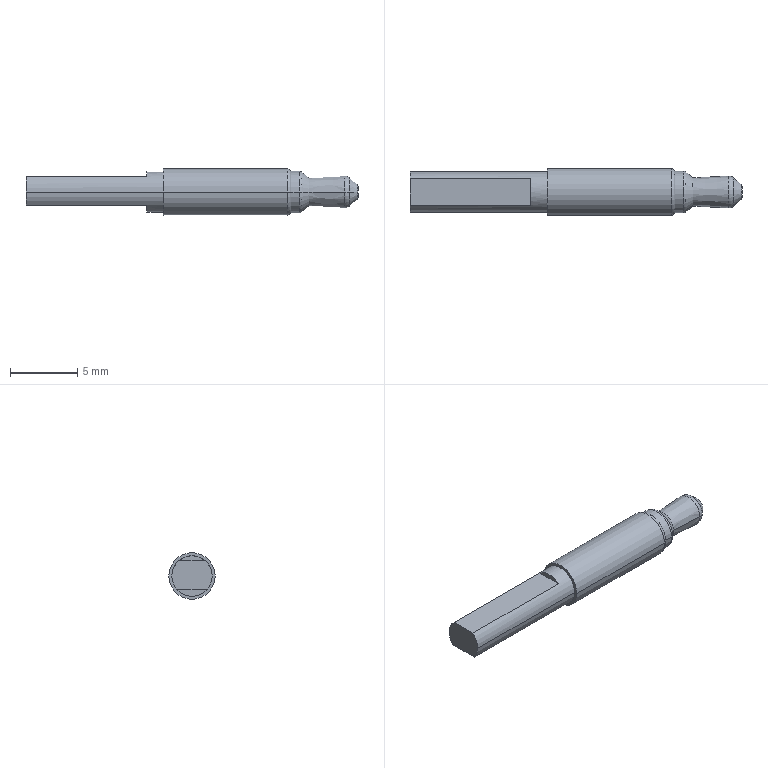Part | NX | 1 solid | 27 faces | box 24.7 x 3.45 x 3.45 mm | volume 170.784 mm3 | torus 8 | plane 7 | cylinder 6 | cone 6 | commonest cylinder face diameters 3 x2 3.1 x2 3.45 x2
STEP:
#1=CARTESIAN_POINT('',(12.641,-1.55,0.));
#2=VERTEX_POINT('',#1);
#3=CARTESIAN_POINT('',(12.641,1.55,0.));
#4=VERTEX_POINT('',#3);
#5=CARTESIAN_POINT('',(12.641,0.,0.));
#6=DIRECTION('',(1.,0.,0.));
#7=DIRECTION('',(0.,-1.,0.));
#8=AXIS2_PLACEMENT_3D('',#5,#6,#7);
#9=CIRCLE('',#8,1.55);
#10=EDGE_CURVE('',#2,#4,#9,.T.);
#11=ORIENTED_EDGE('',*,*,#10,.F.);
#12=CARTESIAN_POINT('',(12.,-1.55,0.));
#13=VERTEX_POINT('',#12);
#14=CARTESIAN_POINT('',(-0.85,-1.55,0.));
#15=DIRECTION('',(1.,0.,0.));
#16=VECTOR('',#15,1000.);
#17=LINE('',#14,#16);
#18=EDGE_CURVE('',#2,#13,#17,.F.);
#19=ORIENTED_EDGE('',*,*,#18,.T.);
#20=CARTESIAN_POINT('',(12.,1.55,0.));
#21=VERTEX_POINT('',#20);
#22=CARTESIAN_POINT('',(12.,0.,0.));
#23=DIRECTION('',(1.,0.,0.));
#24=DIRECTION('',(0.,1.,0.));
#25=AXIS2_PLACEMENT_3D('',#22,#23,#24);
#26=CIRCLE('',#25,1.55);
#27=EDGE_CURVE('',#13,#21,#26,.T.);
#28=ORIENTED_EDGE('',*,*,#27,.T.);
#29=CARTESIAN_POINT('',(-0.85,1.55,0.));
#30=DIRECTION('',(1.,0.,0.));
#31=VECTOR('',#30,1000.);
#32=LINE('',#29,#31);
#33=EDGE_CURVE('',#4,#21,#32,.F.);
#34=ORIENTED_EDGE('',*,*,#33,.F.);
#35=EDGE_LOOP('',(#11,#19,#28,#34));
#36=FACE_BOUND('',#35,.T.);
#37=CARTESIAN_POINT('',(-0.85,0.,0.));
#38=DIRECTION('',(1.,0.,0.));
#39=DIRECTION('',(0.,-1.,0.));
#40=AXIS2_PLACEMENT_3D('',#37,#38,#39);
#41=CYLINDRICAL_SURFACE('',#40,1.55);
#42=ADVANCED_FACE('',(#36),#41,.T.);
#43=CARTESIAN_POINT('',(13.35,-1.05,0.));
#44=VERTEX_POINT('',#43);
#45=CARTESIAN_POINT('',(13.35,1.05,0.));
#46=VERTEX_POINT('',#45);
#47=CARTESIAN_POINT('',(13.35,0.,0.));
#48=DIRECTION('',(1.,0.,0.));
#49=DIRECTION('',(0.,0.,-1.));
#50=AXIS2_PLACEMENT_3D('',#47,#48,#49);
#51=CIRCLE('',#50,1.05);
#52=EDGE_CURVE('',#44,#46,#51,.T.);
#53=ORIENTED_EDGE('',*,*,#52,.F.);
#54=CARTESIAN_POINT('',(12.833,-1.48,0.));
#55=VERTEX_POINT('',#54);
#56=CARTESIAN_POINT('',(13.05,-1.3,0.));
#57=DIRECTION('',(-0.7682,-0.6402,0.));
#58=VECTOR('',#57,1000.);
#59=LINE('',#56,#58);
#60=EDGE_CURVE('',#44,#55,#59,.T.);
#61=ORIENTED_EDGE('',*,*,#60,.T.);
#62=CARTESIAN_POINT('',(12.833,1.48,0.));
#63=VERTEX_POINT('',#62);
#64=CARTESIAN_POINT('',(12.833,0.,0.));
#65=DIRECTION('',(1.,0.,0.));
#66=DIRECTION('',(0.,-1.,0.));
#67=AXIS2_PLACEMENT_3D('',#64,#65,#66);
#68=CIRCLE('',#67,1.48);
#69=EDGE_CURVE('',#55,#63,#68,.T.);
#70=ORIENTED_EDGE('',*,*,#69,.T.);
#71=CARTESIAN_POINT('',(13.05,1.3,0.));
#72=DIRECTION('',(-0.7682,0.6402,0.));
#73=VECTOR('',#72,1000.);
#74=LINE('',#71,#73);
#75=EDGE_CURVE('',#46,#63,#74,.T.);
#76=ORIENTED_EDGE('',*,*,#75,.F.);
#77=EDGE_LOOP('',(#53,#61,#70,#76));
#78=FACE_BOUND('',#77,.T.);
#79=CARTESIAN_POINT('',(13.05,0.,0.));
#80=DIRECTION('',(-1.,0.,0.));
#81=DIRECTION('',(0.,1.,0.));
#82=AXIS2_PLACEMENT_3D('',#79,#80,#81);
#83=CONICAL_SURFACE('',#82,1.3,0.6947);
#84=ADVANCED_FACE('',(#78),#83,.T.);
#85=CARTESIAN_POINT('',(16.932,0.5598,0.));
#86=VERTEX_POINT('',#85);
#87=CARTESIAN_POINT('',(16.932,-0.5598,0.));
#88=VERTEX_POINT('',#87);
#89=CARTESIAN_POINT('',(16.932,0.,0.));
#90=DIRECTION('',(-1.,0.,0.));
#91=DIRECTION('',(0.,-1.,0.));
#92=AXIS2_PLACEMENT_3D('',#89,#90,#91);
#93=CIRCLE('',#92,0.5598);
#94=EDGE_CURVE('',#86,#88,#93,.T.);
#95=ORIENTED_EDGE('',*,*,#94,.T.);
#96=CARTESIAN_POINT('',(16.353,-1.066,0.));
#97=VERTEX_POINT('',#96);
#98=CARTESIAN_POINT('',(16.596,-0.8531,0.));
#99=DIRECTION('',(-0.7526,-0.6585,0.));
#100=VECTOR('',#99,1000.);
#101=LINE('',#98,#100);
#102=EDGE_CURVE('',#88,#97,#101,.T.);
#103=ORIENTED_EDGE('',*,*,#102,.T.);
#104=CARTESIAN_POINT('',(16.353,1.066,0.));
#105=VERTEX_POINT('',#104);
#106=CARTESIAN_POINT('',(16.353,0.,0.));
#107=DIRECTION('',(-1.,0.,0.));
#108=DIRECTION('',(0.,1.,0.));
#109=AXIS2_PLACEMENT_3D('',#106,#107,#108);
#110=CIRCLE('',#109,1.066);
#111=EDGE_CURVE('',#105,#97,#110,.T.);
#112=ORIENTED_EDGE('',*,*,#111,.F.);
#113=CARTESIAN_POINT('',(16.596,0.8531,0.));
#114=DIRECTION('',(-0.7526,0.6585,0.));
#115=VECTOR('',#114,1000.);
#116=LINE('',#113,#115);
#117=EDGE_CURVE('',#86,#105,#116,.T.);
#118=ORIENTED_EDGE('',*,*,#117,.F.);
#119=EDGE_LOOP('',(#95,#103,#112,#118));
#120=FACE_BOUND('',#119,.T.);
#121=CARTESIAN_POINT('',(16.596,0.,0.));
#122=DIRECTION('',(-1.,0.,0.));
#123=DIRECTION('',(0.,1.,0.));
#124=AXIS2_PLACEMENT_3D('',#121,#122,#123);
#125=CONICAL_SURFACE('',#124,0.8531,0.7188);
#126=ADVANCED_FACE('',(#120),#125,.T.);
#127=CARTESIAN_POINT('',(17.,-0.4092,0.));
#128=VERTEX_POINT('',#127);
#129=CARTESIAN_POINT('',(17.,0.4092,0.));
#130=VERTEX_POINT('',#129);
#131=CARTESIAN_POINT('',(17.,0.,0.));
#132=DIRECTION('',(-1.,0.,0.));
#133=DIRECTION('',(0.,1.,0.));
#134=AXIS2_PLACEMENT_3D('',#131,#132,#133);
#135=CIRCLE('',#134,0.4092);
#136=EDGE_CURVE('',#128,#130,#135,.T.);
#137=ORIENTED_EDGE('',*,*,#136,.F.);
#138=CARTESIAN_POINT('',(17.,0.,0.));
#139=DIRECTION('',(-1.,0.,0.));
#140=DIRECTION('',(0.,1.,0.));
#141=AXIS2_PLACEMENT_3D('',#138,#139,#140);
#142=CIRCLE('',#141,0.4092);
#143=EDGE_CURVE('',#130,#128,#142,.T.);
#144=ORIENTED_EDGE('',*,*,#143,.F.);
#145=EDGE_LOOP('',(#137,#144));
#146=FACE_BOUND('',#145,.T.);
#147=CARTESIAN_POINT('',(17.,0.,0.));
#148=DIRECTION('',(1.,0.,0.));
#149=DIRECTION('',(0.,1.,0.));
#150=AXIS2_PLACEMENT_3D('',#147,#148,#149);
#151=PLANE('',#150);
#152=ADVANCED_FACE('',(#146),#151,.T.);
#153=ORIENTED_EDGE('',*,*,#27,.F.);
#154=CARTESIAN_POINT('',(11.727,-1.725,0.));
#155=VERTEX_POINT('',#154);
#156=CARTESIAN_POINT('',(11.727,-1.425,0.));
#157=DIRECTION('',(0.,0.,-1.));
#158=DIRECTION('',(-1.,0.,0.));
#159=AXIS2_PLACEMENT_3D('',#156,#157,#158);
#160=CIRCLE('',#159,0.3);
#161=EDGE_CURVE('',#155,#13,#160,.F.);
#162=ORIENTED_EDGE('',*,*,#161,.F.);
#163=CARTESIAN_POINT('',(11.727,1.725,0.));
#164=VERTEX_POINT('',#163);
#165=CARTESIAN_POINT('',(11.727,0.,0.));
#166=DIRECTION('',(1.,0.,0.));
#167=DIRECTION('',(0.,-1.,0.));
#168=AXIS2_PLACEMENT_3D('',#165,#166,#167);
#169=CIRCLE('',#168,1.725);
#170=EDGE_CURVE('',#155,#164,#169,.T.);
#171=ORIENTED_EDGE('',*,*,#170,.T.);
#172=CARTESIAN_POINT('',(11.727,1.425,0.));
#173=DIRECTION('',(0.,0.,1.));
#174=DIRECTION('',(-1.,0.,0.));
#175=AXIS2_PLACEMENT_3D('',#172,#173,#174);
#176=CIRCLE('',#175,0.3);
#177=EDGE_CURVE('',#164,#21,#176,.F.);
#178=ORIENTED_EDGE('',*,*,#177,.T.);
#179=EDGE_LOOP('',(#153,#162,#171,#178));
#180=FACE_BOUND('',#179,.T.);
#181=CARTESIAN_POINT('',(11.727,0.,0.));
#182=DIRECTION('',(1.,0.,0.));
#183=DIRECTION('',(0.,-1.,0.));
#184=AXIS2_PLACEMENT_3D('',#181,#182,#183);
#185=TOROIDAL_SURFACE('',#184,1.425,0.3);
#186=ADVANCED_FACE('',(#180),#185,.T.);
#187=ORIENTED_EDGE('',*,*,#111,.T.);
#188=CARTESIAN_POINT('',(15.997,-1.189,0.));
#189=VERTEX_POINT('',#188);
#190=CARTESIAN_POINT('',(16.024,-0.69,0.));
#191=DIRECTION('',(0.,0.,1.));
#192=DIRECTION('',(-1.,0.,0.));
#193=AXIS2_PLACEMENT_3D('',#190,#191,#192);
#194=CIRCLE('',#193,0.5);
#195=EDGE_CURVE('',#189,#97,#194,.T.);
#196=ORIENTED_EDGE('',*,*,#195,.F.);
#197=CARTESIAN_POINT('',(15.997,1.189,0.));
#198=VERTEX_POINT('',#197);
#199=CARTESIAN_POINT('',(15.997,0.,0.));
#200=DIRECTION('',(-1.,0.,0.));
#201=DIRECTION('',(0.,1.,0.));
#202=AXIS2_PLACEMENT_3D('',#199,#200,#201);
#203=CIRCLE('',#202,1.189);
#204=EDGE_CURVE('',#198,#189,#203,.T.);
#205=ORIENTED_EDGE('',*,*,#204,.F.);
#206=CARTESIAN_POINT('',(16.024,0.69,0.));
#207=DIRECTION('',(0.,0.,-1.));
#208=DIRECTION('',(-1.,0.,0.));
#209=AXIS2_PLACEMENT_3D('',#206,#207,#208);
#210=CIRCLE('',#209,0.5);
#211=EDGE_CURVE('',#198,#105,#210,.T.);
#212=ORIENTED_EDGE('',*,*,#211,.T.);
#213=EDGE_LOOP('',(#187,#196,#205,#212));
#214=FACE_BOUND('',#213,.T.);
#215=CARTESIAN_POINT('',(16.024,0.,0.));
#216=DIRECTION('',(-1.,0.,0.));
#217=DIRECTION('',(0.,1.,0.));
#218=AXIS2_PLACEMENT_3D('',#215,#216,#217);
#219=TOROIDAL_SURFACE('',#218,0.69,0.5);
#220=ADVANCED_FACE('',(#214),#219,.T.);
#221=CARTESIAN_POINT('',(2.5,1.725,0.));
#222=VERTEX_POINT('',#221);
#223=CARTESIAN_POINT('',(2.5,-1.725,0.));
#224=VERTEX_POINT('',#223);
#225=CARTESIAN_POINT('',(2.5,0.,0.));
#226=DIRECTION('',(1.,0.,0.));
#227=DIRECTION('',(0.,-1.,0.));
#228=AXIS2_PLACEMENT_3D('',#225,#226,#227);
#229=CIRCLE('',#228,1.725);
#230=EDGE_CURVE('',#222,#224,#229,.T.);
#231=ORIENTED_EDGE('',*,*,#230,.T.);
#232=CARTESIAN_POINT('',(0.,-1.725,0.));
#233=DIRECTION('',(1.,0.,0.));
#234=VECTOR('',#233,1000.);
#235=LINE('',#232,#234);
#236=EDGE_CURVE('',#155,#224,#235,.F.);
#237=ORIENTED_EDGE('',*,*,#236,.F.);
#238=CARTESIAN_POINT('',(11.727,0.,0.));
#239=DIRECTION('',(1.,0.,0.));
#240=DIRECTION('',(0.,-1.,0.));
#241=AXIS2_PLACEMENT_3D('',#238,#239,#240);
#242=CIRCLE('',#241,1.725);
#243=EDGE_CURVE('',#164,#155,#242,.T.);
#244=ORIENTED_EDGE('',*,*,#243,.F.);
#245=CARTESIAN_POINT('',(0.,1.725,0.));
#246=DIRECTION('',(1.,0.,0.));
#247=VECTOR('',#246,1000.);
#248=LINE('',#245,#247);
#249=EDGE_CURVE('',#164,#222,#248,.F.);
#250=ORIENTED_EDGE('',*,*,#249,.T.);
#251=EDGE_LOOP('',(#231,#237,#244,#250));
#252=FACE_BOUND('',#251,.T.);
#253=CARTESIAN_POINT('',(0.,0.,0.));
#254=DIRECTION('',(1.,0.,0.));
#255=DIRECTION('',(0.,-1.,0.));
#256=AXIS2_PLACEMENT_3D('',#253,#254,#255);
#257=CYLINDRICAL_SURFACE('',#256,1.725);
#258=ADVANCED_FACE('',(#252),#257,.T.);
#259=ORIENTED_EDGE('',*,*,#204,.T.);
#260=CARTESIAN_POINT('',(14.734,-1.123,0.));
#261=DIRECTION('',(0.9986,-0.05256,0.));
#262=VECTOR('',#261,1000.);
#263=LINE('',#260,#262);
#264=EDGE_CURVE('',#189,#44,#263,.F.);
#265=ORIENTED_EDGE('',*,*,#264,.T.);
#266=ORIENTED_EDGE('',*,*,#52,.T.);
#267=CARTESIAN_POINT('',(14.734,1.123,0.));
#268=DIRECTION('',(0.9986,0.05256,0.));
#269=VECTOR('',#268,1000.);
#270=LINE('',#267,#269);
#271=EDGE_CURVE('',#198,#46,#270,.F.);
#272=ORIENTED_EDGE('',*,*,#271,.F.);
#273=EDGE_LOOP('',(#259,#265,#266,#272));
#274=FACE_BOUND('',#273,.T.);
#275=CARTESIAN_POINT('',(14.734,0.,0.));
#276=DIRECTION('',(1.,0.,0.));
#277=DIRECTION('',(0.,-1.,0.));
#278=AXIS2_PLACEMENT_3D('',#275,#276,#277);
#279=CONICAL_SURFACE('',#278,1.123,0.05258);
#280=ADVANCED_FACE('',(#274),#279,.T.);
#281=ORIENTED_EDGE('',*,*,#10,.T.);
#282=CARTESIAN_POINT('',(12.641,1.25,0.));
#283=DIRECTION('',(0.,0.,1.));
#284=DIRECTION('',(-1.,0.,0.));
#285=AXIS2_PLACEMENT_3D('',#282,#283,#284);
#286=CIRCLE('',#285,0.3);
#287=EDGE_CURVE('',#4,#63,#286,.F.);
#288=ORIENTED_EDGE('',*,*,#287,.T.);
#289=ORIENTED_EDGE('',*,*,#69,.F.);
#290=CARTESIAN_POINT('',(12.641,-1.25,0.));
#291=DIRECTION('',(0.,0.,-1.));
#292=DIRECTION('',(-1.,0.,0.));
#293=AXIS2_PLACEMENT_3D('',#290,#291,#292);
#294=CIRCLE('',#293,0.3);
#295=EDGE_CURVE('',#2,#55,#294,.F.);
#296=ORIENTED_EDGE('',*,*,#295,.F.);
#297=EDGE_LOOP('',(#281,#288,#289,#296));
#298=FACE_BOUND('',#297,.T.);
#299=CARTESIAN_POINT('',(12.641,0.,0.));
#300=DIRECTION('',(1.,0.,0.));
#301=DIRECTION('',(0.,-1.,0.));
#302=AXIS2_PLACEMENT_3D('',#299,#300,#301);
#303=TOROIDAL_SURFACE('',#302,1.25,0.3);
#304=ADVANCED_FACE('',(#298),#303,.T.);
#305=ORIENTED_EDGE('',*,*,#136,.T.);
#306=CARTESIAN_POINT('',(16.8,0.4092,0.));
#307=DIRECTION('',(0.,0.,1.));
#308=DIRECTION('',(-1.,0.,0.));
#309=AXIS2_PLACEMENT_3D('',#306,#307,#308);
#310=CIRCLE('',#309,0.2);
#311=EDGE_CURVE('',#130,#86,#310,.T.);
#312=ORIENTED_EDGE('',*,*,#311,.T.);
#313=CARTESIAN_POINT('',(16.932,0.,0.));
#314=DIRECTION('',(-1.,0.,0.));
#315=DIRECTION('',(0.,-1.,0.));
#316=AXIS2_PLACEMENT_3D('',#313,#314,#315);
#317=CIRCLE('',#316,0.5598);
#318=EDGE_CURVE('',#88,#86,#317,.T.);
#319=ORIENTED_EDGE('',*,*,#318,.F.);
#320=CARTESIAN_POINT('',(16.8,-0.4092,0.));
#321=DIRECTION('',(0.,0.,-1.));
#322=DIRECTION('',(-1.,0.,0.));
#323=AXIS2_PLACEMENT_3D('',#320,#321,#322);
#324=CIRCLE('',#323,0.2);
#325=EDGE_CURVE('',#128,#88,#324,.T.);
#326=ORIENTED_EDGE('',*,*,#325,.F.);
#327=EDGE_LOOP('',(#305,#312,#319,#326));
#328=FACE_BOUND('',#327,.T.);
#329=CARTESIAN_POINT('',(16.8,0.,0.));
#330=DIRECTION('',(1.,0.,0.));
#331=DIRECTION('',(0.,-1.,0.));
#332=AXIS2_PLACEMENT_3D('',#329,#330,#331);
#333=TOROIDAL_SURFACE('',#332,0.4092,0.2);
#334=ADVANCED_FACE('',(#328),#333,.T.);
#335=ORIENTED_EDGE('',*,*,#230,.F.);
#336=CARTESIAN_POINT('',(2.5,0.,0.));
#337=DIRECTION('',(1.,0.,0.));
#338=DIRECTION('',(0.,-1.,0.));
#339=AXIS2_PLACEMENT_3D('',#336,#337,#338);
#340=CIRCLE('',#339,1.725);
#341=EDGE_CURVE('',#224,#222,#340,.T.);
#342=ORIENTED_EDGE('',*,*,#341,.F.);
#343=EDGE_LOOP('',(#335,#342));
#344=FACE_BOUND('',#343,.T.);
#345=CARTESIAN_POINT('',(2.5,1.5,0.));
#346=VERTEX_POINT('',#345);
#347=CARTESIAN_POINT('',(2.5,-1.5,0.));
#348=VERTEX_POINT('',#347);
#349=CARTESIAN_POINT('',(2.5,0.,0.));
#350=DIRECTION('',(-1.,0.,0.));
#351=DIRECTION('',(0.,-1.,0.));
#352=AXIS2_PLACEMENT_3D('',#349,#350,#351);
#353=CIRCLE('',#352,1.5);
#354=EDGE_CURVE('',#346,#348,#353,.T.);
#355=ORIENTED_EDGE('',*,*,#354,.F.);
#356=CARTESIAN_POINT('',(2.5,0.,0.));
#357=DIRECTION('',(-1.,0.,0.));
#358=DIRECTION('',(0.,-1.,0.));
#359=AXIS2_PLACEMENT_3D('',#356,#357,#358);
#360=CIRCLE('',#359,1.5);
#361=EDGE_CURVE('',#348,#346,#360,.T.);
#362=ORIENTED_EDGE('',*,*,#361,.F.);
#363=EDGE_LOOP('',(#355,#362));
#364=FACE_BOUND('',#363,.T.);
#365=CARTESIAN_POINT('',(2.5,-28.452,3.6));
#366=DIRECTION('',(1.,0.,0.));
#367=DIRECTION('',(0.,0.,1.));
#368=AXIS2_PLACEMENT_3D('',#365,#366,#367);
#369=PLANE('',#368);
#370=ADVANCED_FACE('',(#344,#364),#369,.F.);
#371=CARTESIAN_POINT('',(-7.7,1.5,0.));
#372=VERTEX_POINT('',#371);
#373=CARTESIAN_POINT('',(-7.7,1.144,-0.97));
#374=VERTEX_POINT('',#373);
#375=CARTESIAN_POINT('',(-7.7,0.,0.));
#376=DIRECTION('',(-1.,0.,0.));
#377=DIRECTION('',(0.,-1.,0.));
#378=AXIS2_PLACEMENT_3D('',#375,#376,#377);
#379=CIRCLE('',#378,1.5);
#380=EDGE_CURVE('',#372,#374,#379,.T.);
#381=ORIENTED_EDGE('',*,*,#380,.F.);
#382=CARTESIAN_POINT('',(2.3,1.5,0.));
#383=DIRECTION('',(-1.,0.,0.));
#384=VECTOR('',#383,1000.);
#385=LINE('',#382,#384);
#386=EDGE_CURVE('',#372,#346,#385,.F.);
#387=ORIENTED_EDGE('',*,*,#386,.T.);
#388=ORIENTED_EDGE('',*,*,#354,.T.);
#389=CARTESIAN_POINT('',(-7.7,-1.5,0.));
#390=VERTEX_POINT('',#389);
#391=CARTESIAN_POINT('',(2.3,-1.5,0.));
#392=DIRECTION('',(-1.,0.,0.));
#393=VECTOR('',#392,1000.);
#394=LINE('',#391,#393);
#395=EDGE_CURVE('',#390,#348,#394,.F.);
#396=ORIENTED_EDGE('',*,*,#395,.F.);
#397=CARTESIAN_POINT('',(-7.7,-1.144,-0.97));
#398=VERTEX_POINT('',#397);
#399=CARTESIAN_POINT('',(-7.7,0.,0.));
#400=DIRECTION('',(-1.,0.,0.));
#401=DIRECTION('',(0.,-1.,0.));
#402=AXIS2_PLACEMENT_3D('',#399,#400,#401);
#403=CIRCLE('',#402,1.5);
#404=EDGE_CURVE('',#398,#390,#403,.T.);
#405=ORIENTED_EDGE('',*,*,#404,.F.);
#406=CARTESIAN_POINT('',(1.3,-1.144,-0.97));
#407=VERTEX_POINT('',#406);
#408=CARTESIAN_POINT('',(2.3,-1.144,-0.97));
#409=DIRECTION('',(-1.,0.,0.));
#410=VECTOR('',#409,1000.);
#411=LINE('',#408,#410);
#412=EDGE_CURVE('',#398,#407,#411,.F.);
#413=ORIENTED_EDGE('',*,*,#412,.T.);
#414=CARTESIAN_POINT('',(1.3,1.144,-0.97));
#415=VERTEX_POINT('',#414);
#416=CARTESIAN_POINT('',(1.3,0.,0.));
#417=DIRECTION('',(-1.,0.,0.));
#418=DIRECTION('',(0.,-1.,0.));
#419=AXIS2_PLACEMENT_3D('',#416,#417,#418);
#420=CIRCLE('',#419,1.5);
#421=EDGE_CURVE('',#415,#407,#420,.T.);
#422=ORIENTED_EDGE('',*,*,#421,.F.);
#423=CARTESIAN_POINT('',(2.3,1.144,-0.97));
#424=DIRECTION('',(-1.,0.,0.));
#425=VECTOR('',#424,1000.);
#426=LINE('',#423,#425);
#427=EDGE_CURVE('',#374,#415,#426,.F.);
#428=ORIENTED_EDGE('',*,*,#427,.F.);
#429=EDGE_LOOP('',(#381,#387,#388,#396,#405,#413,#422,#428));
#430=FACE_BOUND('',#429,.T.);
#431=CARTESIAN_POINT('',(2.3,0.,0.));
#432=DIRECTION('',(-1.,0.,0.));
#433=DIRECTION('',(0.,-1.,0.));
#434=AXIS2_PLACEMENT_3D('',#431,#432,#433);
#435=CYLINDRICAL_SURFACE('',#434,1.5);
#436=ADVANCED_FACE('',(#430),#435,.T.);
#437=ORIENTED_EDGE('',*,*,#380,.T.);
#438=CARTESIAN_POINT('',(-7.7,0.,-0.97));
#439=DIRECTION('',(0.,1.,0.));
#440=VECTOR('',#439,1000.);
#441=LINE('',#438,#440);
#442=EDGE_CURVE('',#398,#374,#441,.T.);
#443=ORIENTED_EDGE('',*,*,#442,.F.);
#444=ORIENTED_EDGE('',*,*,#404,.T.);
#445=CARTESIAN_POINT('',(-7.7,-0.9864,1.13));
#446=VERTEX_POINT('',#445);
#447=CARTESIAN_POINT('',(-7.7,0.,0.));
#448=DIRECTION('',(-1.,0.,0.));
#449=DIRECTION('',(0.,-1.,0.));
#450=AXIS2_PLACEMENT_3D('',#447,#448,#449);
#451=CIRCLE('',#450,1.5);
#452=EDGE_CURVE('',#390,#446,#451,.T.);
#453=ORIENTED_EDGE('',*,*,#452,.T.);
#454=CARTESIAN_POINT('',(-7.7,0.9864,1.13));
#455=VERTEX_POINT('',#454);
#456=CARTESIAN_POINT('',(-7.7,0.,1.13));
#457=DIRECTION('',(0.,-1.,0.));
#458=VECTOR('',#457,1000.);
#459=LINE('',#456,#458);
#460=EDGE_CURVE('',#455,#446,#459,.T.);
#461=ORIENTED_EDGE('',*,*,#460,.F.);
#462=CARTESIAN_POINT('',(-7.7,0.,0.));
#463=DIRECTION('',(-1.,0.,0.));
#464=DIRECTION('',(0.,-1.,0.));
#465=AXIS2_PLACEMENT_3D('',#462,#463,#464);
#466=CIRCLE('',#465,1.5);
#467=EDGE_CURVE('',#455,#372,#466,.T.);
#468=ORIENTED_EDGE('',*,*,#467,.T.);
#469=EDGE_LOOP('',(#437,#443,#444,#453,#461,#468));
#470=FACE_BOUND('',#469,.T.);
#471=CARTESIAN_POINT('',(-7.7,0.6142,-0.2899));
#472=DIRECTION('',(-1.,0.,0.));
#473=DIRECTION('',(0.,0.,1.));
#474=AXIS2_PLACEMENT_3D('',#471,#472,#473);
#475=PLANE('',#474);
#476=ADVANCED_FACE('',(#470),#475,.T.);
#477=ORIENTED_EDGE('',*,*,#421,.T.);
#478=CARTESIAN_POINT('',(1.3,-1.5,-0.97));
#479=DIRECTION('',(0.,1.,0.));
#480=VECTOR('',#479,1000.);
#481=LINE('',#478,#480);
#482=EDGE_CURVE('',#407,#415,#481,.T.);
#483=ORIENTED_EDGE('',*,*,#482,.T.);
#484=EDGE_LOOP('',(#477,#483));
#485=FACE_BOUND('',#484,.T.);
#486=CARTESIAN_POINT('',(1.3,1.5,-2.47));
#487=DIRECTION('',(1.,0.,0.));
#488=DIRECTION('',(0.,0.,1.));
#489=AXIS2_PLACEMENT_3D('',#486,#487,#488);
#490=PLANE('',#489);
#491=ADVANCED_FACE('',(#485),#490,.F.);
#492=ORIENTED_EDGE('',*,*,#412,.F.);
#493=ORIENTED_EDGE('',*,*,#442,.T.);
#494=ORIENTED_EDGE('',*,*,#427,.T.);
#495=ORIENTED_EDGE('',*,*,#482,.F.);
#496=EDGE_LOOP('',(#492,#493,#494,#495));
#497=FACE_BOUND('',#496,.T.);
#498=CARTESIAN_POINT('',(-3.393,-0.2163,-0.97));
#499=DIRECTION('',(0.,0.,-1.));
#500=DIRECTION('',(0.,-1.,0.));
#501=AXIS2_PLACEMENT_3D('',#498,#499,#500);
#502=PLANE('',#501);
#503=ADVANCED_FACE('',(#497),#502,.T.);
#504=CARTESIAN_POINT('',(1.3,-0.9864,1.13));
#505=VERTEX_POINT('',#504);
#506=CARTESIAN_POINT('',(1.3,0.9864,1.13));
#507=VERTEX_POINT('',#506);
#508=CARTESIAN_POINT('',(1.3,0.,0.));
#509=DIRECTION('',(-1.,0.,0.));
#510=DIRECTION('',(0.,-1.,0.));
#511=AXIS2_PLACEMENT_3D('',#508,#509,#510);
#512=CIRCLE('',#511,1.5);
#513=EDGE_CURVE('',#505,#507,#512,.T.);
#514=ORIENTED_EDGE('',*,*,#513,.T.);
#515=CARTESIAN_POINT('',(1.3,-5.456,1.13));
#516=DIRECTION('',(0.,1.,0.));
#517=VECTOR('',#516,1000.);
#518=LINE('',#515,#517);
#519=EDGE_CURVE('',#505,#507,#518,.T.);
#520=ORIENTED_EDGE('',*,*,#519,.F.);
#521=EDGE_LOOP('',(#514,#520));
#522=FACE_BOUND('',#521,.T.);
#523=CARTESIAN_POINT('',(1.3,-5.456,3.53));
#524=DIRECTION('',(1.,0.,0.));
#525=DIRECTION('',(0.,1.,0.));
#526=AXIS2_PLACEMENT_3D('',#523,#524,#525);
#527=PLANE('',#526);
#528=ADVANCED_FACE('',(#522),#527,.F.);
#529=CARTESIAN_POINT('',(2.3,0.9864,1.13));
#530=DIRECTION('',(-1.,0.,0.));
#531=VECTOR('',#530,1000.);
#532=LINE('',#529,#531);
#533=EDGE_CURVE('',#507,#455,#532,.T.);
#534=ORIENTED_EDGE('',*,*,#533,.T.);
#535=ORIENTED_EDGE('',*,*,#460,.T.);
#536=CARTESIAN_POINT('',(2.3,-0.9864,1.13));
#537=DIRECTION('',(-1.,0.,0.));
#538=VECTOR('',#537,1000.);
#539=LINE('',#536,#538);
#540=EDGE_CURVE('',#505,#446,#539,.T.);
#541=ORIENTED_EDGE('',*,*,#540,.F.);
#542=ORIENTED_EDGE('',*,*,#519,.T.);
#543=EDGE_LOOP('',(#534,#535,#541,#542));
#544=FACE_BOUND('',#543,.T.);
#545=CARTESIAN_POINT('',(-5.112,-0.01314,1.13));
#546=DIRECTION('',(0.,0.,1.));
#547=DIRECTION('',(1.,0.,0.));
#548=AXIS2_PLACEMENT_3D('',#545,#546,#547);
#549=PLANE('',#548);
#550=ADVANCED_FACE('',(#544),#549,.T.);
#551=ORIENTED_EDGE('',*,*,#18,.F.);
#552=CARTESIAN_POINT('',(12.641,0.,0.));
#553=DIRECTION('',(1.,0.,0.));
#554=DIRECTION('',(0.,-1.,0.));
#555=AXIS2_PLACEMENT_3D('',#552,#553,#554);
#556=CIRCLE('',#555,1.55);
#557=EDGE_CURVE('',#4,#2,#556,.T.);
#558=ORIENTED_EDGE('',*,*,#557,.F.);
#559=ORIENTED_EDGE('',*,*,#33,.T.);
#560=CARTESIAN_POINT('',(12.,0.,0.));
#561=DIRECTION('',(1.,0.,0.));
#562=DIRECTION('',(0.,1.,0.));
#563=AXIS2_PLACEMENT_3D('',#560,#561,#562);
#564=CIRCLE('',#563,1.55);
#565=EDGE_CURVE('',#21,#13,#564,.T.);
#566=ORIENTED_EDGE('',*,*,#565,.T.);
#567=EDGE_LOOP('',(#551,#558,#559,#566));
#568=FACE_BOUND('',#567,.T.);
#569=CARTESIAN_POINT('',(-0.85,0.,0.));
#570=DIRECTION('',(1.,0.,0.));
#571=DIRECTION('',(0.,-1.,0.));
#572=AXIS2_PLACEMENT_3D('',#569,#570,#571);
#573=CYLINDRICAL_SURFACE('',#572,1.55);
#574=ADVANCED_FACE('',(#568),#573,.T.);
#575=ORIENTED_EDGE('',*,*,#264,.F.);
#576=CARTESIAN_POINT('',(15.997,0.,0.));
#577=DIRECTION('',(-1.,0.,0.));
#578=DIRECTION('',(0.,1.,0.));
#579=AXIS2_PLACEMENT_3D('',#576,#577,#578);
#580=CIRCLE('',#579,1.189);
#581=EDGE_CURVE('',#189,#198,#580,.T.);
#582=ORIENTED_EDGE('',*,*,#581,.T.);
#583=ORIENTED_EDGE('',*,*,#271,.T.);
#584=CARTESIAN_POINT('',(13.35,0.,0.));
#585=DIRECTION('',(1.,0.,0.));
#586=DIRECTION('',(0.,0.,-1.));
#587=AXIS2_PLACEMENT_3D('',#584,#585,#586);
#588=CIRCLE('',#587,1.05);
#589=EDGE_CURVE('',#46,#44,#588,.T.);
#590=ORIENTED_EDGE('',*,*,#589,.T.);
#591=EDGE_LOOP('',(#575,#582,#583,#590));
#592=FACE_BOUND('',#591,.T.);
#593=CARTESIAN_POINT('',(14.734,0.,0.));
#594=DIRECTION('',(1.,0.,0.));
#595=DIRECTION('',(0.,-1.,0.));
#596=AXIS2_PLACEMENT_3D('',#593,#594,#595);
#597=CONICAL_SURFACE('',#596,1.123,0.05258);
#598=ADVANCED_FACE('',(#592),#597,.T.);
#599=ORIENTED_EDGE('',*,*,#395,.T.);
#600=ORIENTED_EDGE('',*,*,#361,.T.);
#601=ORIENTED_EDGE('',*,*,#386,.F.);
#602=ORIENTED_EDGE('',*,*,#467,.F.);
#603=ORIENTED_EDGE('',*,*,#533,.F.);
#604=ORIENTED_EDGE('',*,*,#513,.F.);
#605=ORIENTED_EDGE('',*,*,#540,.T.);
#606=ORIENTED_EDGE('',*,*,#452,.F.);
#607=EDGE_LOOP('',(#599,#600,#601,#602,#603,#604,#605,#606));
#608=FACE_BOUND('',#607,.T.);
#609=CARTESIAN_POINT('',(2.3,0.,0.));
#610=DIRECTION('',(-1.,0.,0.));
#611=DIRECTION('',(0.,-1.,0.));
#612=AXIS2_PLACEMENT_3D('',#609,#610,#611);
#613=CYLINDRICAL_SURFACE('',#612,1.5);
#614=ADVANCED_FACE('',(#608),#613,.T.);
#615=ORIENTED_EDGE('',*,*,#236,.T.);
#616=ORIENTED_EDGE('',*,*,#341,.T.);
#617=ORIENTED_EDGE('',*,*,#249,.F.);
#618=ORIENTED_EDGE('',*,*,#170,.F.);
#619=EDGE_LOOP('',(#615,#616,#617,#618));
#620=FACE_BOUND('',#619,.T.);
#621=CARTESIAN_POINT('',(0.,0.,0.));
#622=DIRECTION('',(1.,0.,0.));
#623=DIRECTION('',(0.,-1.,0.));
#624=AXIS2_PLACEMENT_3D('',#621,#622,#623);
#625=CYLINDRICAL_SURFACE('',#624,1.725);
#626=ADVANCED_FACE('',(#620),#625,.T.);
#627=ORIENTED_EDGE('',*,*,#117,.T.);
#628=CARTESIAN_POINT('',(16.353,0.,0.));
#629=DIRECTION('',(-1.,0.,0.));
#630=DIRECTION('',(0.,1.,0.));
#631=AXIS2_PLACEMENT_3D('',#628,#629,#630);
#632=CIRCLE('',#631,1.066);
#633=EDGE_CURVE('',#97,#105,#632,.T.);
#634=ORIENTED_EDGE('',*,*,#633,.F.);
#635=ORIENTED_EDGE('',*,*,#102,.F.);
#636=ORIENTED_EDGE('',*,*,#318,.T.);
#637=EDGE_LOOP('',(#627,#634,#635,#636));
#638=FACE_BOUND('',#637,.T.);
#639=CARTESIAN_POINT('',(16.596,0.,0.));
#640=DIRECTION('',(-1.,0.,0.));
#641=DIRECTION('',(0.,1.,0.));
#642=AXIS2_PLACEMENT_3D('',#639,#640,#641);
#643=CONICAL_SURFACE('',#642,0.8531,0.7188);
#644=ADVANCED_FACE('',(#638),#643,.T.);
#645=ORIENTED_EDGE('',*,*,#75,.T.);
#646=CARTESIAN_POINT('',(12.833,0.,0.));
#647=DIRECTION('',(1.,0.,0.));
#648=DIRECTION('',(0.,-1.,0.));
#649=AXIS2_PLACEMENT_3D('',#646,#647,#648);
#650=CIRCLE('',#649,1.48);
#651=EDGE_CURVE('',#63,#55,#650,.T.);
#652=ORIENTED_EDGE('',*,*,#651,.T.);
#653=ORIENTED_EDGE('',*,*,#60,.F.);
#654=ORIENTED_EDGE('',*,*,#589,.F.);
#655=EDGE_LOOP('',(#645,#652,#653,#654));
#656=FACE_BOUND('',#655,.T.);
#657=CARTESIAN_POINT('',(13.05,0.,0.));
#658=DIRECTION('',(-1.,0.,0.));
#659=DIRECTION('',(0.,1.,0.));
#660=AXIS2_PLACEMENT_3D('',#657,#658,#659);
#661=CONICAL_SURFACE('',#660,1.3,0.6947);
#662=ADVANCED_FACE('',(#656),#661,.T.);
#663=ORIENTED_EDGE('',*,*,#94,.F.);
#664=ORIENTED_EDGE('',*,*,#311,.F.);
#665=ORIENTED_EDGE('',*,*,#143,.T.);
#666=ORIENTED_EDGE('',*,*,#325,.T.);
#667=EDGE_LOOP('',(#663,#664,#665,#666));
#668=FACE_BOUND('',#667,.T.);
#669=CARTESIAN_POINT('',(16.8,0.,0.));
#670=DIRECTION('',(1.,0.,0.));
#671=DIRECTION('',(0.,-1.,0.));
#672=AXIS2_PLACEMENT_3D('',#669,#670,#671);
#673=TOROIDAL_SURFACE('',#672,0.4092,0.2);
#674=ADVANCED_FACE('',(#668),#673,.T.);
#675=ORIENTED_EDGE('',*,*,#243,.T.);
#676=ORIENTED_EDGE('',*,*,#161,.T.);
#677=ORIENTED_EDGE('',*,*,#565,.F.);
#678=ORIENTED_EDGE('',*,*,#177,.F.);
#679=EDGE_LOOP('',(#675,#676,#677,#678));
#680=FACE_BOUND('',#679,.T.);
#681=CARTESIAN_POINT('',(11.727,0.,0.));
#682=DIRECTION('',(1.,0.,0.));
#683=DIRECTION('',(0.,-1.,0.));
#684=AXIS2_PLACEMENT_3D('',#681,#682,#683);
#685=TOROIDAL_SURFACE('',#684,1.425,0.3);
#686=ADVANCED_FACE('',(#680),#685,.T.);
#687=ORIENTED_EDGE('',*,*,#211,.F.);
#688=ORIENTED_EDGE('',*,*,#581,.F.);
#689=ORIENTED_EDGE('',*,*,#195,.T.);
#690=ORIENTED_EDGE('',*,*,#633,.T.);
#691=EDGE_LOOP('',(#687,#688,#689,#690));
#692=FACE_BOUND('',#691,.T.);
#693=CARTESIAN_POINT('',(16.024,0.,0.));
#694=DIRECTION('',(-1.,0.,0.));
#695=DIRECTION('',(0.,1.,0.));
#696=AXIS2_PLACEMENT_3D('',#693,#694,#695);
#697=TOROIDAL_SURFACE('',#696,0.69,0.5);
#698=ADVANCED_FACE('',(#692),#697,.T.);
#699=ORIENTED_EDGE('',*,*,#295,.T.);
#700=ORIENTED_EDGE('',*,*,#651,.F.);
#701=ORIENTED_EDGE('',*,*,#287,.F.);
#702=ORIENTED_EDGE('',*,*,#557,.T.);
#703=EDGE_LOOP('',(#699,#700,#701,#702));
#704=FACE_BOUND('',#703,.T.);
#705=CARTESIAN_POINT('',(12.641,0.,0.));
#706=DIRECTION('',(1.,0.,0.));
#707=DIRECTION('',(0.,-1.,0.));
#708=AXIS2_PLACEMENT_3D('',#705,#706,#707);
#709=TOROIDAL_SURFACE('',#708,1.25,0.3);
#710=ADVANCED_FACE('',(#704),#709,.T.);
#711=CLOSED_SHELL('',(#42,#84,#126,#152,#186,#220,#258,#280,#304,#334,#370,#436,#476,#491,#503,#528,#550,#574,#598,#614,#626,#644,#662,#674,#686,#698,#710));
#712=MANIFOLD_SOLID_BREP('',#711);
#713=(LENGTH_UNIT()NAMED_UNIT(*)SI_UNIT(.MILLI.,.METRE.));
#714=UNCERTAINTY_MEASURE_WITH_UNIT(LENGTH_MEASURE(0.00001),#713,'','');
#715=(NAMED_UNIT(*)PLANE_ANGLE_UNIT()SI_UNIT($,.RADIAN.));
#716=(NAMED_UNIT(*)SI_UNIT($,.STERADIAN.)SOLID_ANGLE_UNIT());
#717=(GEOMETRIC_REPRESENTATION_CONTEXT(3)GLOBAL_UNCERTAINTY_ASSIGNED_CONTEXT((#714))GLOBAL_UNIT_ASSIGNED_CONTEXT((#713,#715,#716))REPRESENTATION_CONTEXT('',''));
#718=ADVANCED_BREP_SHAPE_REPRESENTATION('',(#712),#717);